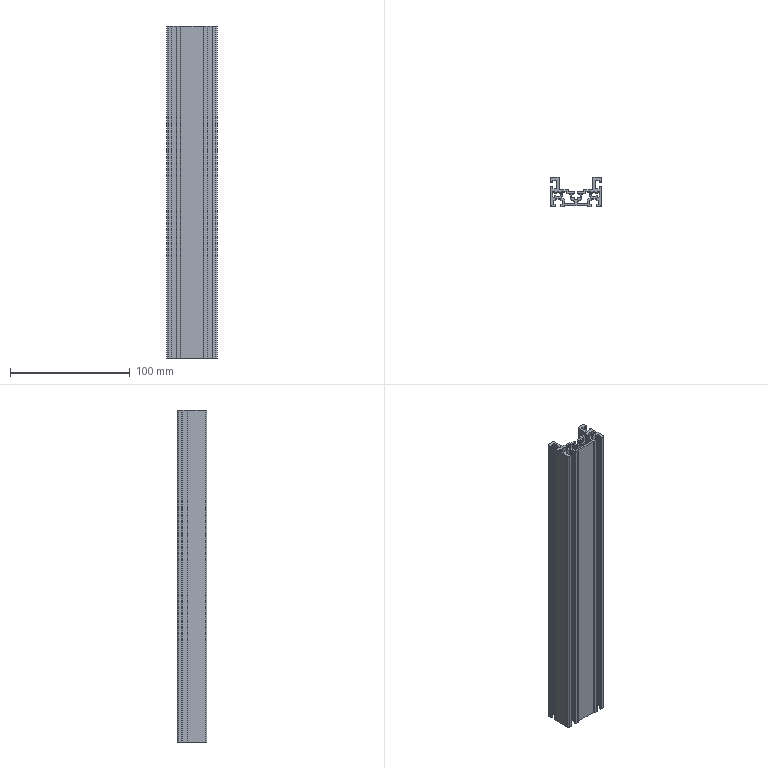Part | SolidWorks | features Extrusion 1, WeldmentFeature 1 | 1 solid | 213 faces | box 42 x 24.4 x 277 mm | volume 94986 mm3 | cylinder 117 | plane 96 | commonest cylinder face diameters 0.6 x84 1 x8 2 x6 1.026 x4 1.719 x4 4.2 x4